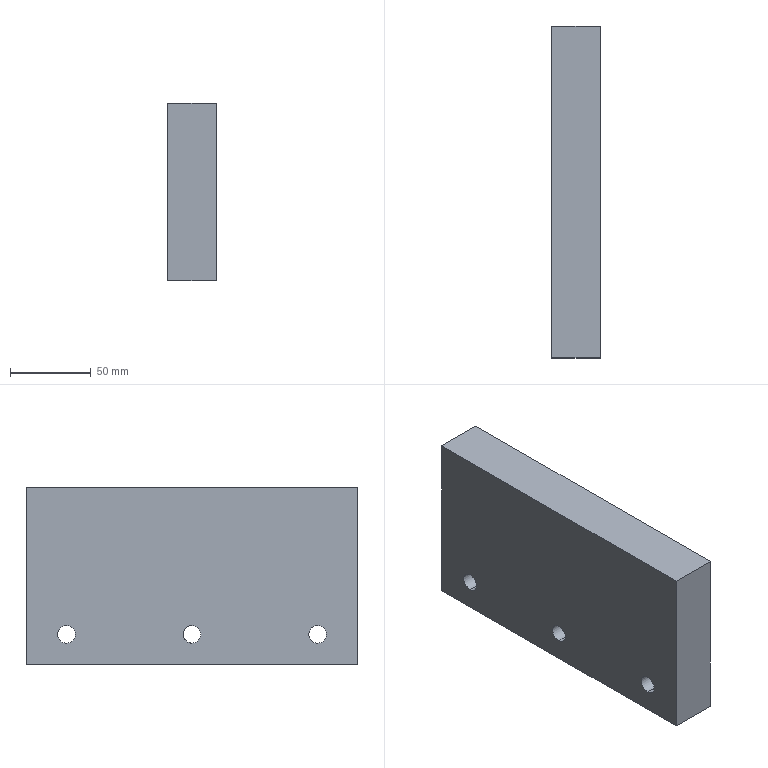Part | Creo | 1 solid | 21 faces | box 30 x 206.013 x 110.125 mm | volume 667483 mm3 | cylinder 12 | plane 9 | commonest cylinder face diameters 11 x6 17.25 x6
STEP:
#1=CARTESIAN_POINT('',(0.,0.,0.));
#2=DIRECTION('',(0.,0.,1.));
#3=DIRECTION('',(1.,0.,0.));
#4=AXIS2_PLACEMENT_3D('',#1,#2,#3);
#5=CARTESIAN_POINT('',(798.101,-95.244,-43.317));
#6=VERTEX_POINT('',#5);
#7=CARTESIAN_POINT('',(798.101,110.769,-43.317));
#8=VERTEX_POINT('',#7);
#9=CARTESIAN_POINT('',(798.101,-95.244,-43.317));
#10=DIRECTION('',(0.,1.,0.));
#11=VECTOR('',#10,206.013);
#12=LINE('',#9,#11);
#13=EDGE_CURVE('',#6,#8,#12,.T.);
#14=ORIENTED_EDGE('',*,*,#13,.T.);
#15=CARTESIAN_POINT('',(798.101,110.769,-153.441));
#16=VERTEX_POINT('',#15);
#17=CARTESIAN_POINT('',(798.101,110.769,-43.317));
#18=DIRECTION('',(0.,0.,-1.));
#19=VECTOR('',#18,110.125);
#20=LINE('',#17,#19);
#21=EDGE_CURVE('',#8,#16,#20,.T.);
#22=ORIENTED_EDGE('',*,*,#21,.T.);
#23=CARTESIAN_POINT('',(798.101,-95.244,-153.441));
#24=VERTEX_POINT('',#23);
#25=CARTESIAN_POINT('',(798.101,-95.244,-153.441));
#26=DIRECTION('',(0.,1.,0.));
#27=VECTOR('',#26,206.013);
#28=LINE('',#25,#27);
#29=EDGE_CURVE('',#24,#16,#28,.T.);
#30=ORIENTED_EDGE('',*,*,#29,.F.);
#31=CARTESIAN_POINT('',(798.101,-95.244,-43.317));
#32=DIRECTION('',(0.,0.,-1.));
#33=VECTOR('',#32,110.125);
#34=LINE('',#31,#33);
#35=EDGE_CURVE('',#6,#24,#34,.T.);
#36=ORIENTED_EDGE('',*,*,#35,.F.);
#37=EDGE_LOOP('',(#14,#22,#30,#36));
#38=FACE_OUTER_BOUND('',#37,.F.);
#39=CARTESIAN_POINT('',(798.101,16.387,-134.619));
#40=VERTEX_POINT('',#39);
#41=CARTESIAN_POINT('',(798.101,7.762,-143.244));
#42=VERTEX_POINT('',#41);
#43=CARTESIAN_POINT('',(798.101,7.762,-134.619));
#44=DIRECTION('',(-1.,0.,0.));
#45=DIRECTION('',(0.,1.,0.));
#46=AXIS2_PLACEMENT_3D('',#43,#44,#45);
#47=CIRCLE('',#46,8.625);
#48=EDGE_CURVE('',#40,#42,#47,.T.);
#49=ORIENTED_EDGE('',*,*,#48,.F.);
#50=CARTESIAN_POINT('',(798.101,7.762,-125.994));
#51=VERTEX_POINT('',#50);
#52=CARTESIAN_POINT('',(798.101,7.762,-134.619));
#53=DIRECTION('',(-1.,0.,0.));
#54=DIRECTION('',(0.,0.,1.));
#55=AXIS2_PLACEMENT_3D('',#52,#53,#54);
#56=CIRCLE('',#55,8.625);
#57=EDGE_CURVE('',#51,#40,#56,.T.);
#58=ORIENTED_EDGE('',*,*,#57,.F.);
#59=CARTESIAN_POINT('',(798.101,7.762,-134.619));
#60=DIRECTION('',(-1.,0.,0.));
#61=DIRECTION('',(0.,0.,-1.));
#62=AXIS2_PLACEMENT_3D('',#59,#60,#61);
#63=CIRCLE('',#62,8.625);
#64=EDGE_CURVE('',#42,#51,#63,.T.);
#65=ORIENTED_EDGE('',*,*,#64,.F.);
#66=EDGE_LOOP('',(#49,#58,#65));
#67=FACE_BOUND('',#66,.F.);
#68=CARTESIAN_POINT('',(798.101,94.394,-134.619));
#69=VERTEX_POINT('',#68);
#70=CARTESIAN_POINT('',(798.101,85.769,-143.244));
#71=VERTEX_POINT('',#70);
#72=CARTESIAN_POINT('',(798.101,85.769,-134.619));
#73=DIRECTION('',(-1.,0.,0.));
#74=DIRECTION('',(0.,1.,0.));
#75=AXIS2_PLACEMENT_3D('',#72,#73,#74);
#76=CIRCLE('',#75,8.625);
#77=EDGE_CURVE('',#69,#71,#76,.T.);
#78=ORIENTED_EDGE('',*,*,#77,.F.);
#79=CARTESIAN_POINT('',(798.101,85.769,-125.994));
#80=VERTEX_POINT('',#79);
#81=CARTESIAN_POINT('',(798.101,85.769,-134.619));
#82=DIRECTION('',(-1.,0.,0.));
#83=DIRECTION('',(0.,0.,1.));
#84=AXIS2_PLACEMENT_3D('',#81,#82,#83);
#85=CIRCLE('',#84,8.625);
#86=EDGE_CURVE('',#80,#69,#85,.T.);
#87=ORIENTED_EDGE('',*,*,#86,.F.);
#88=CARTESIAN_POINT('',(798.101,85.769,-134.619));
#89=DIRECTION('',(-1.,0.,0.));
#90=DIRECTION('',(0.,0.,-1.));
#91=AXIS2_PLACEMENT_3D('',#88,#89,#90);
#92=CIRCLE('',#91,8.625);
#93=EDGE_CURVE('',#71,#80,#92,.T.);
#94=ORIENTED_EDGE('',*,*,#93,.F.);
#95=EDGE_LOOP('',(#78,#87,#94));
#96=FACE_BOUND('',#95,.F.);
#97=CARTESIAN_POINT('',(798.101,-61.619,-134.619));
#98=VERTEX_POINT('',#97);
#99=CARTESIAN_POINT('',(798.101,-70.244,-143.244));
#100=VERTEX_POINT('',#99);
#101=CARTESIAN_POINT('',(798.101,-70.244,-134.619));
#102=DIRECTION('',(-1.,0.,0.));
#103=DIRECTION('',(0.,1.,0.));
#104=AXIS2_PLACEMENT_3D('',#101,#102,#103);
#105=CIRCLE('',#104,8.625);
#106=EDGE_CURVE('',#98,#100,#105,.T.);
#107=ORIENTED_EDGE('',*,*,#106,.F.);
#108=CARTESIAN_POINT('',(798.101,-70.244,-125.994));
#109=VERTEX_POINT('',#108);
#110=CARTESIAN_POINT('',(798.101,-70.244,-134.619));
#111=DIRECTION('',(-1.,0.,0.));
#112=DIRECTION('',(0.,0.,1.));
#113=AXIS2_PLACEMENT_3D('',#110,#111,#112);
#114=CIRCLE('',#113,8.625);
#115=EDGE_CURVE('',#109,#98,#114,.T.);
#116=ORIENTED_EDGE('',*,*,#115,.F.);
#117=CARTESIAN_POINT('',(798.101,-70.244,-134.619));
#118=DIRECTION('',(-1.,0.,0.));
#119=DIRECTION('',(0.,0.,-1.));
#120=AXIS2_PLACEMENT_3D('',#117,#118,#119);
#121=CIRCLE('',#120,8.625);
#122=EDGE_CURVE('',#100,#109,#121,.T.);
#123=ORIENTED_EDGE('',*,*,#122,.F.);
#124=EDGE_LOOP('',(#107,#116,#123));
#125=FACE_BOUND('',#124,.F.);
#126=CARTESIAN_POINT('',(798.101,8.76,-121.835));
#127=DIRECTION('',(-1.,0.,0.));
#128=DIRECTION('',(0.,0.,1.));
#129=AXIS2_PLACEMENT_3D('',#126,#127,#128);
#130=PLANE('',#129);
#131=ADVANCED_FACE('',(#38,#67,#96,#125),#130,.F.);
#132=ORIENTED_EDGE('',*,*,#57,.T.);
#133=ORIENTED_EDGE('',*,*,#48,.T.);
#134=CARTESIAN_POINT('',(787.101,7.762,-143.244));
#135=VERTEX_POINT('',#134);
#136=CARTESIAN_POINT('',(787.101,7.762,-143.244));
#137=DIRECTION('',(1.,0.,0.));
#138=VECTOR('',#137,11.);
#139=LINE('',#136,#138);
#140=EDGE_CURVE('',#135,#42,#139,.T.);
#141=ORIENTED_EDGE('',*,*,#140,.F.);
#142=CARTESIAN_POINT('',(787.101,16.387,-134.619));
#143=VERTEX_POINT('',#142);
#144=CARTESIAN_POINT('',(787.101,7.762,-134.619));
#145=DIRECTION('',(1.,0.,0.));
#146=DIRECTION('',(0.,0.,-1.));
#147=AXIS2_PLACEMENT_3D('',#144,#145,#146);
#148=CIRCLE('',#147,8.625);
#149=EDGE_CURVE('',#135,#143,#148,.T.);
#150=ORIENTED_EDGE('',*,*,#149,.T.);
#151=CARTESIAN_POINT('',(787.101,7.762,-125.994));
#152=VERTEX_POINT('',#151);
#153=CARTESIAN_POINT('',(787.101,7.762,-134.619));
#154=DIRECTION('',(1.,0.,0.));
#155=DIRECTION('',(0.,1.,0.));
#156=AXIS2_PLACEMENT_3D('',#153,#154,#155);
#157=CIRCLE('',#156,8.625);
#158=EDGE_CURVE('',#143,#152,#157,.T.);
#159=ORIENTED_EDGE('',*,*,#158,.T.);
#160=CARTESIAN_POINT('',(787.101,7.762,-125.994));
#161=DIRECTION('',(1.,0.,0.));
#162=VECTOR('',#161,11.);
#163=LINE('',#160,#162);
#164=EDGE_CURVE('',#152,#51,#163,.T.);
#165=ORIENTED_EDGE('',*,*,#164,.T.);
#166=EDGE_LOOP('',(#132,#133,#141,#150,#159,#165));
#167=FACE_OUTER_BOUND('',#166,.F.);
#168=CARTESIAN_POINT('',(787.101,7.762,-134.619));
#169=DIRECTION('',(1.,0.,0.));
#170=DIRECTION('',(0.,0.,-1.));
#171=AXIS2_PLACEMENT_3D('',#168,#169,#170);
#172=CYLINDRICAL_SURFACE('',#171,8.625);
#173=ADVANCED_FACE('',(#167),#172,.F.);
#174=ORIENTED_EDGE('',*,*,#64,.T.);
#175=ORIENTED_EDGE('',*,*,#164,.F.);
#176=CARTESIAN_POINT('',(787.101,-0.8626,-134.619));
#177=VERTEX_POINT('',#176);
#178=CARTESIAN_POINT('',(787.101,7.762,-134.619));
#179=DIRECTION('',(1.,0.,0.));
#180=DIRECTION('',(0.,0.,1.));
#181=AXIS2_PLACEMENT_3D('',#178,#179,#180);
#182=CIRCLE('',#181,8.625);
#183=EDGE_CURVE('',#152,#177,#182,.T.);
#184=ORIENTED_EDGE('',*,*,#183,.T.);
#185=CARTESIAN_POINT('',(787.101,7.762,-134.619));
#186=DIRECTION('',(1.,0.,0.));
#187=DIRECTION('',(0.,-1.,0.));
#188=AXIS2_PLACEMENT_3D('',#185,#186,#187);
#189=CIRCLE('',#188,8.625);
#190=EDGE_CURVE('',#177,#135,#189,.T.);
#191=ORIENTED_EDGE('',*,*,#190,.T.);
#192=ORIENTED_EDGE('',*,*,#140,.T.);
#193=EDGE_LOOP('',(#174,#175,#184,#191,#192));
#194=FACE_OUTER_BOUND('',#193,.F.);
#195=CARTESIAN_POINT('',(787.101,7.762,-134.619));
#196=DIRECTION('',(1.,0.,0.));
#197=DIRECTION('',(0.,0.,-1.));
#198=AXIS2_PLACEMENT_3D('',#195,#196,#197);
#199=CYLINDRICAL_SURFACE('',#198,8.625);
#200=ADVANCED_FACE('',(#194),#199,.F.);
#201=ORIENTED_EDGE('',*,*,#158,.F.);
#202=ORIENTED_EDGE('',*,*,#149,.F.);
#203=ORIENTED_EDGE('',*,*,#190,.F.);
#204=ORIENTED_EDGE('',*,*,#183,.F.);
#205=EDGE_LOOP('',(#201,#202,#203,#204));
#206=FACE_OUTER_BOUND('',#205,.F.);
#207=CARTESIAN_POINT('',(787.101,2.262,-134.619));
#208=VERTEX_POINT('',#207);
#209=CARTESIAN_POINT('',(787.101,7.762,-129.119));
#210=VERTEX_POINT('',#209);
#211=CARTESIAN_POINT('',(787.101,7.762,-134.619));
#212=DIRECTION('',(-1.,0.,0.));
#213=DIRECTION('',(0.,-1.,0.));
#214=AXIS2_PLACEMENT_3D('',#211,#212,#213);
#215=CIRCLE('',#214,5.5);
#216=EDGE_CURVE('',#208,#210,#215,.T.);
#217=ORIENTED_EDGE('',*,*,#216,.F.);
#218=CARTESIAN_POINT('',(787.101,7.762,-140.119));
#219=VERTEX_POINT('',#218);
#220=CARTESIAN_POINT('',(787.101,7.762,-134.619));
#221=DIRECTION('',(-1.,0.,0.));
#222=DIRECTION('',(0.,0.,-1.));
#223=AXIS2_PLACEMENT_3D('',#220,#221,#222);
#224=CIRCLE('',#223,5.5);
#225=EDGE_CURVE('',#219,#208,#224,.T.);
#226=ORIENTED_EDGE('',*,*,#225,.F.);
#227=CARTESIAN_POINT('',(787.101,13.262,-134.619));
#228=VERTEX_POINT('',#227);
#229=CARTESIAN_POINT('',(787.101,7.762,-134.619));
#230=DIRECTION('',(-1.,0.,0.));
#231=DIRECTION('',(0.,1.,0.));
#232=AXIS2_PLACEMENT_3D('',#229,#230,#231);
#233=CIRCLE('',#232,5.5);
#234=EDGE_CURVE('',#228,#219,#233,.T.);
#235=ORIENTED_EDGE('',*,*,#234,.F.);
#236=CARTESIAN_POINT('',(787.101,7.762,-134.619));
#237=DIRECTION('',(-1.,0.,0.));
#238=DIRECTION('',(0.,0.,1.));
#239=AXIS2_PLACEMENT_3D('',#236,#237,#238);
#240=CIRCLE('',#239,5.5);
#241=EDGE_CURVE('',#210,#228,#240,.T.);
#242=ORIENTED_EDGE('',*,*,#241,.F.);
#243=EDGE_LOOP('',(#217,#226,#235,#242));
#244=FACE_BOUND('',#243,.F.);
#245=CARTESIAN_POINT('',(787.101,7.762,-134.619));
#246=DIRECTION('',(-1.,0.,0.));
#247=DIRECTION('',(0.,0.,1.));
#248=AXIS2_PLACEMENT_3D('',#245,#246,#247);
#249=PLANE('',#248);
#250=ADVANCED_FACE('',(#206,#244),#249,.F.);
#251=CARTESIAN_POINT('',(768.101,7.762,-129.119));
#252=VERTEX_POINT('',#251);
#253=CARTESIAN_POINT('',(768.101,2.262,-134.619));
#254=VERTEX_POINT('',#253);
#255=CARTESIAN_POINT('',(768.101,7.762,-134.619));
#256=DIRECTION('',(1.,0.,0.));
#257=DIRECTION('',(0.,0.,1.));
#258=AXIS2_PLACEMENT_3D('',#255,#256,#257);
#259=CIRCLE('',#258,5.5);
#260=EDGE_CURVE('',#252,#254,#259,.T.);
#261=ORIENTED_EDGE('',*,*,#260,.T.);
#262=CARTESIAN_POINT('',(768.101,7.762,-140.119));
#263=VERTEX_POINT('',#262);
#264=CARTESIAN_POINT('',(768.101,7.762,-134.619));
#265=DIRECTION('',(1.,0.,0.));
#266=DIRECTION('',(0.,-1.,0.));
#267=AXIS2_PLACEMENT_3D('',#264,#265,#266);
#268=CIRCLE('',#267,5.5);
#269=EDGE_CURVE('',#254,#263,#268,.T.);
#270=ORIENTED_EDGE('',*,*,#269,.T.);
#271=CARTESIAN_POINT('',(787.101,7.762,-140.119));
#272=DIRECTION('',(-1.,0.,0.));
#273=VECTOR('',#272,19.);
#274=LINE('',#271,#273);
#275=EDGE_CURVE('',#219,#263,#274,.T.);
#276=ORIENTED_EDGE('',*,*,#275,.F.);
#277=ORIENTED_EDGE('',*,*,#225,.T.);
#278=ORIENTED_EDGE('',*,*,#216,.T.);
#279=CARTESIAN_POINT('',(787.101,7.762,-129.119));
#280=DIRECTION('',(-1.,0.,0.));
#281=VECTOR('',#280,19.);
#282=LINE('',#279,#281);
#283=EDGE_CURVE('',#210,#252,#282,.T.);
#284=ORIENTED_EDGE('',*,*,#283,.T.);
#285=EDGE_LOOP('',(#261,#270,#276,#277,#278,#284));
#286=FACE_OUTER_BOUND('',#285,.F.);
#287=CARTESIAN_POINT('',(787.101,7.762,-134.619));
#288=DIRECTION('',(-1.,0.,0.));
#289=DIRECTION('',(0.,0.,1.));
#290=AXIS2_PLACEMENT_3D('',#287,#288,#289);
#291=CYLINDRICAL_SURFACE('',#290,5.5);
#292=ADVANCED_FACE('',(#286),#291,.F.);
#293=CARTESIAN_POINT('',(768.101,-95.244,-43.317));
#294=VERTEX_POINT('',#293);
#295=CARTESIAN_POINT('',(768.101,-95.244,-153.441));
#296=VERTEX_POINT('',#295);
#297=CARTESIAN_POINT('',(768.101,-95.244,-43.317));
#298=DIRECTION('',(0.,0.,-1.));
#299=VECTOR('',#298,110.125);
#300=LINE('',#297,#299);
#301=EDGE_CURVE('',#294,#296,#300,.T.);
#302=ORIENTED_EDGE('',*,*,#301,.T.);
#303=CARTESIAN_POINT('',(768.101,110.769,-153.441));
#304=VERTEX_POINT('',#303);
#305=CARTESIAN_POINT('',(768.101,-95.244,-153.441));
#306=DIRECTION('',(0.,1.,0.));
#307=VECTOR('',#306,206.013);
#308=LINE('',#305,#307);
#309=EDGE_CURVE('',#296,#304,#308,.T.);
#310=ORIENTED_EDGE('',*,*,#309,.T.);
#311=CARTESIAN_POINT('',(768.101,110.769,-43.317));
#312=VERTEX_POINT('',#311);
#313=CARTESIAN_POINT('',(768.101,110.769,-43.317));
#314=DIRECTION('',(0.,0.,-1.));
#315=VECTOR('',#314,110.125);
#316=LINE('',#313,#315);
#317=EDGE_CURVE('',#312,#304,#316,.T.);
#318=ORIENTED_EDGE('',*,*,#317,.F.);
#319=CARTESIAN_POINT('',(768.101,-95.244,-43.317));
#320=DIRECTION('',(0.,1.,0.));
#321=VECTOR('',#320,206.013);
#322=LINE('',#319,#321);
#323=EDGE_CURVE('',#294,#312,#322,.T.);
#324=ORIENTED_EDGE('',*,*,#323,.F.);
#325=EDGE_LOOP('',(#302,#310,#318,#324));
#326=FACE_OUTER_BOUND('',#325,.F.);
#327=ORIENTED_EDGE('',*,*,#269,.F.);
#328=ORIENTED_EDGE('',*,*,#260,.F.);
#329=CARTESIAN_POINT('',(768.101,7.762,-134.619));
#330=DIRECTION('',(1.,0.,0.));
#331=DIRECTION('',(0.,0.,-1.));
#332=AXIS2_PLACEMENT_3D('',#329,#330,#331);
#333=CIRCLE('',#332,5.5);
#334=EDGE_CURVE('',#263,#252,#333,.T.);
#335=ORIENTED_EDGE('',*,*,#334,.F.);
#336=EDGE_LOOP('',(#327,#328,#335));
#337=FACE_BOUND('',#336,.F.);
#338=CARTESIAN_POINT('',(768.101,80.269,-134.619));
#339=VERTEX_POINT('',#338);
#340=CARTESIAN_POINT('',(768.101,85.769,-140.119));
#341=VERTEX_POINT('',#340);
#342=CARTESIAN_POINT('',(768.101,85.769,-134.619));
#343=DIRECTION('',(1.,0.,0.));
#344=DIRECTION('',(0.,-1.,0.));
#345=AXIS2_PLACEMENT_3D('',#342,#343,#344);
#346=CIRCLE('',#345,5.5);
#347=EDGE_CURVE('',#339,#341,#346,.T.);
#348=ORIENTED_EDGE('',*,*,#347,.F.);
#349=CARTESIAN_POINT('',(768.101,85.769,-129.119));
#350=VERTEX_POINT('',#349);
#351=CARTESIAN_POINT('',(768.101,85.769,-134.619));
#352=DIRECTION('',(1.,0.,0.));
#353=DIRECTION('',(0.,0.,1.));
#354=AXIS2_PLACEMENT_3D('',#351,#352,#353);
#355=CIRCLE('',#354,5.5);
#356=EDGE_CURVE('',#350,#339,#355,.T.);
#357=ORIENTED_EDGE('',*,*,#356,.F.);
#358=CARTESIAN_POINT('',(768.101,85.769,-134.619));
#359=DIRECTION('',(1.,0.,0.));
#360=DIRECTION('',(0.,0.,-1.));
#361=AXIS2_PLACEMENT_3D('',#358,#359,#360);
#362=CIRCLE('',#361,5.5);
#363=EDGE_CURVE('',#341,#350,#362,.T.);
#364=ORIENTED_EDGE('',*,*,#363,.F.);
#365=EDGE_LOOP('',(#348,#357,#364));
#366=FACE_BOUND('',#365,.F.);
#367=CARTESIAN_POINT('',(768.101,-75.744,-134.619));
#368=VERTEX_POINT('',#367);
#369=CARTESIAN_POINT('',(768.101,-70.244,-140.119));
#370=VERTEX_POINT('',#369);
#371=CARTESIAN_POINT('',(768.101,-70.244,-134.619));
#372=DIRECTION('',(1.,0.,0.));
#373=DIRECTION('',(0.,-1.,0.));
#374=AXIS2_PLACEMENT_3D('',#371,#372,#373);
#375=CIRCLE('',#374,5.5);
#376=EDGE_CURVE('',#368,#370,#375,.T.);
#377=ORIENTED_EDGE('',*,*,#376,.F.);
#378=CARTESIAN_POINT('',(768.101,-70.244,-129.119));
#379=VERTEX_POINT('',#378);
#380=CARTESIAN_POINT('',(768.101,-70.244,-134.619));
#381=DIRECTION('',(1.,0.,0.));
#382=DIRECTION('',(0.,0.,1.));
#383=AXIS2_PLACEMENT_3D('',#380,#381,#382);
#384=CIRCLE('',#383,5.5);
#385=EDGE_CURVE('',#379,#368,#384,.T.);
#386=ORIENTED_EDGE('',*,*,#385,.F.);
#387=CARTESIAN_POINT('',(768.101,-70.244,-134.619));
#388=DIRECTION('',(1.,0.,0.));
#389=DIRECTION('',(0.,0.,-1.));
#390=AXIS2_PLACEMENT_3D('',#387,#388,#389);
#391=CIRCLE('',#390,5.5);
#392=EDGE_CURVE('',#370,#379,#391,.T.);
#393=ORIENTED_EDGE('',*,*,#392,.F.);
#394=EDGE_LOOP('',(#377,#386,#393));
#395=FACE_BOUND('',#394,.F.);
#396=CARTESIAN_POINT('',(768.101,8.76,-121.835));
#397=DIRECTION('',(-1.,0.,0.));
#398=DIRECTION('',(0.,0.,1.));
#399=AXIS2_PLACEMENT_3D('',#396,#397,#398);
#400=PLANE('',#399);
#401=ADVANCED_FACE('',(#326,#337,#366,#395),#400,.T.);
#402=ORIENTED_EDGE('',*,*,#385,.T.);
#403=ORIENTED_EDGE('',*,*,#376,.T.);
#404=CARTESIAN_POINT('',(787.101,-70.244,-140.119));
#405=VERTEX_POINT('',#404);
#406=CARTESIAN_POINT('',(787.101,-70.244,-140.119));
#407=DIRECTION('',(-1.,0.,0.));
#408=VECTOR('',#407,19.);
#409=LINE('',#406,#408);
#410=EDGE_CURVE('',#405,#370,#409,.T.);
#411=ORIENTED_EDGE('',*,*,#410,.F.);
#412=CARTESIAN_POINT('',(787.101,-75.744,-134.619));
#413=VERTEX_POINT('',#412);
#414=CARTESIAN_POINT('',(787.101,-70.244,-134.619));
#415=DIRECTION('',(-1.,0.,0.));
#416=DIRECTION('',(0.,0.,-1.));
#417=AXIS2_PLACEMENT_3D('',#414,#415,#416);
#418=CIRCLE('',#417,5.5);
#419=EDGE_CURVE('',#405,#413,#418,.T.);
#420=ORIENTED_EDGE('',*,*,#419,.T.);
#421=CARTESIAN_POINT('',(787.101,-70.244,-129.119));
#422=VERTEX_POINT('',#421);
#423=CARTESIAN_POINT('',(787.101,-70.244,-134.619));
#424=DIRECTION('',(-1.,0.,0.));
#425=DIRECTION('',(0.,-1.,0.));
#426=AXIS2_PLACEMENT_3D('',#423,#424,#425);
#427=CIRCLE('',#426,5.5);
#428=EDGE_CURVE('',#413,#422,#427,.T.);
#429=ORIENTED_EDGE('',*,*,#428,.T.);
#430=CARTESIAN_POINT('',(787.101,-70.244,-129.119));
#431=DIRECTION('',(-1.,0.,0.));
#432=VECTOR('',#431,19.);
#433=LINE('',#430,#432);
#434=EDGE_CURVE('',#422,#379,#433,.T.);
#435=ORIENTED_EDGE('',*,*,#434,.T.);
#436=EDGE_LOOP('',(#402,#403,#411,#420,#429,#435));
#437=FACE_OUTER_BOUND('',#436,.F.);
#438=CARTESIAN_POINT('',(787.101,-70.244,-134.619));
#439=DIRECTION('',(-1.,0.,0.));
#440=DIRECTION('',(0.,0.,1.));
#441=AXIS2_PLACEMENT_3D('',#438,#439,#440);
#442=CYLINDRICAL_SURFACE('',#441,5.5);
#443=ADVANCED_FACE('',(#437),#442,.F.);
#444=ORIENTED_EDGE('',*,*,#392,.T.);
#445=ORIENTED_EDGE('',*,*,#434,.F.);
#446=CARTESIAN_POINT('',(787.101,-64.744,-134.619));
#447=VERTEX_POINT('',#446);
#448=CARTESIAN_POINT('',(787.101,-70.244,-134.619));
#449=DIRECTION('',(-1.,0.,0.));
#450=DIRECTION('',(0.,0.,1.));
#451=AXIS2_PLACEMENT_3D('',#448,#449,#450);
#452=CIRCLE('',#451,5.5);
#453=EDGE_CURVE('',#422,#447,#452,.T.);
#454=ORIENTED_EDGE('',*,*,#453,.T.);
#455=CARTESIAN_POINT('',(787.101,-70.244,-134.619));
#456=DIRECTION('',(-1.,0.,0.));
#457=DIRECTION('',(0.,1.,0.));
#458=AXIS2_PLACEMENT_3D('',#455,#456,#457);
#459=CIRCLE('',#458,5.5);
#460=EDGE_CURVE('',#447,#405,#459,.T.);
#461=ORIENTED_EDGE('',*,*,#460,.T.);
#462=ORIENTED_EDGE('',*,*,#410,.T.);
#463=EDGE_LOOP('',(#444,#445,#454,#461,#462));
#464=FACE_OUTER_BOUND('',#463,.F.);
#465=CARTESIAN_POINT('',(787.101,-70.244,-134.619));
#466=DIRECTION('',(-1.,0.,0.));
#467=DIRECTION('',(0.,0.,1.));
#468=AXIS2_PLACEMENT_3D('',#465,#466,#467);
#469=CYLINDRICAL_SURFACE('',#468,5.5);
#470=ADVANCED_FACE('',(#464),#469,.F.);
#471=CARTESIAN_POINT('',(787.101,-61.619,-134.619));
#472=VERTEX_POINT('',#471);
#473=CARTESIAN_POINT('',(787.101,-70.244,-125.994));
#474=VERTEX_POINT('',#473);
#475=CARTESIAN_POINT('',(787.101,-70.244,-134.619));
#476=DIRECTION('',(1.,0.,0.));
#477=DIRECTION('',(0.,1.,0.));
#478=AXIS2_PLACEMENT_3D('',#475,#476,#477);
#479=CIRCLE('',#478,8.625);
#480=EDGE_CURVE('',#472,#474,#479,.T.);
#481=ORIENTED_EDGE('',*,*,#480,.F.);
#482=CARTESIAN_POINT('',(787.101,-70.244,-143.244));
#483=VERTEX_POINT('',#482);
#484=CARTESIAN_POINT('',(787.101,-70.244,-134.619));
#485=DIRECTION('',(1.,0.,0.));
#486=DIRECTION('',(0.,0.,-1.));
#487=AXIS2_PLACEMENT_3D('',#484,#485,#486);
#488=CIRCLE('',#487,8.625);
#489=EDGE_CURVE('',#483,#472,#488,.T.);
#490=ORIENTED_EDGE('',*,*,#489,.F.);
#491=CARTESIAN_POINT('',(787.101,-78.869,-134.619));
#492=VERTEX_POINT('',#491);
#493=CARTESIAN_POINT('',(787.101,-70.244,-134.619));
#494=DIRECTION('',(1.,0.,0.));
#495=DIRECTION('',(0.,-1.,0.));
#496=AXIS2_PLACEMENT_3D('',#493,#494,#495);
#497=CIRCLE('',#496,8.625);
#498=EDGE_CURVE('',#492,#483,#497,.T.);
#499=ORIENTED_EDGE('',*,*,#498,.F.);
#500=CARTESIAN_POINT('',(787.101,-70.244,-134.619));
#501=DIRECTION('',(1.,0.,0.));
#502=DIRECTION('',(0.,0.,1.));
#503=AXIS2_PLACEMENT_3D('',#500,#501,#502);
#504=CIRCLE('',#503,8.625);
#505=EDGE_CURVE('',#474,#492,#504,.T.);
#506=ORIENTED_EDGE('',*,*,#505,.F.);
#507=EDGE_LOOP('',(#481,#490,#499,#506));
#508=FACE_OUTER_BOUND('',#507,.F.);
#509=ORIENTED_EDGE('',*,*,#428,.F.);
#510=ORIENTED_EDGE('',*,*,#419,.F.);
#511=ORIENTED_EDGE('',*,*,#460,.F.);
#512=ORIENTED_EDGE('',*,*,#453,.F.);
#513=EDGE_LOOP('',(#509,#510,#511,#512));
#514=FACE_BOUND('',#513,.F.);
#515=CARTESIAN_POINT('',(787.101,-70.244,-134.619));
#516=DIRECTION('',(-1.,0.,0.));
#517=DIRECTION('',(0.,0.,1.));
#518=AXIS2_PLACEMENT_3D('',#515,#516,#517);
#519=PLANE('',#518);
#520=ADVANCED_FACE('',(#508,#514),#519,.F.);
#521=ORIENTED_EDGE('',*,*,#115,.T.);
#522=ORIENTED_EDGE('',*,*,#106,.T.);
#523=CARTESIAN_POINT('',(787.101,-70.244,-143.244));
#524=DIRECTION('',(1.,0.,0.));
#525=VECTOR('',#524,11.);
#526=LINE('',#523,#525);
#527=EDGE_CURVE('',#483,#100,#526,.T.);
#528=ORIENTED_EDGE('',*,*,#527,.F.);
#529=ORIENTED_EDGE('',*,*,#489,.T.);
#530=ORIENTED_EDGE('',*,*,#480,.T.);
#531=CARTESIAN_POINT('',(787.101,-70.244,-125.994));
#532=DIRECTION('',(1.,0.,0.));
#533=VECTOR('',#532,11.);
#534=LINE('',#531,#533);
#535=EDGE_CURVE('',#474,#109,#534,.T.);
#536=ORIENTED_EDGE('',*,*,#535,.T.);
#537=EDGE_LOOP('',(#521,#522,#528,#529,#530,#536));
#538=FACE_OUTER_BOUND('',#537,.F.);
#539=CARTESIAN_POINT('',(787.101,-70.244,-134.619));
#540=DIRECTION('',(1.,0.,0.));
#541=DIRECTION('',(0.,0.,-1.));
#542=AXIS2_PLACEMENT_3D('',#539,#540,#541);
#543=CYLINDRICAL_SURFACE('',#542,8.625);
#544=ADVANCED_FACE('',(#538),#543,.F.);
#545=ORIENTED_EDGE('',*,*,#122,.T.);
#546=ORIENTED_EDGE('',*,*,#535,.F.);
#547=ORIENTED_EDGE('',*,*,#505,.T.);
#548=ORIENTED_EDGE('',*,*,#498,.T.);
#549=ORIENTED_EDGE('',*,*,#527,.T.);
#550=EDGE_LOOP('',(#545,#546,#547,#548,#549));
#551=FACE_OUTER_BOUND('',#550,.F.);
#552=CARTESIAN_POINT('',(787.101,-70.244,-134.619));
#553=DIRECTION('',(1.,0.,0.));
#554=DIRECTION('',(0.,0.,-1.));
#555=AXIS2_PLACEMENT_3D('',#552,#553,#554);
#556=CYLINDRICAL_SURFACE('',#555,8.625);
#557=ADVANCED_FACE('',(#551),#556,.F.);
#558=ORIENTED_EDGE('',*,*,#334,.T.);
#559=ORIENTED_EDGE('',*,*,#283,.F.);
#560=ORIENTED_EDGE('',*,*,#241,.T.);
#561=ORIENTED_EDGE('',*,*,#234,.T.);
#562=ORIENTED_EDGE('',*,*,#275,.T.);
#563=EDGE_LOOP('',(#558,#559,#560,#561,#562));
#564=FACE_OUTER_BOUND('',#563,.F.);
#565=CARTESIAN_POINT('',(787.101,7.762,-134.619));
#566=DIRECTION('',(-1.,0.,0.));
#567=DIRECTION('',(0.,0.,1.));
#568=AXIS2_PLACEMENT_3D('',#565,#566,#567);
#569=CYLINDRICAL_SURFACE('',#568,5.5);
#570=ADVANCED_FACE('',(#564),#569,.F.);
#571=ORIENTED_EDGE('',*,*,#356,.T.);
#572=ORIENTED_EDGE('',*,*,#347,.T.);
#573=CARTESIAN_POINT('',(787.101,85.769,-140.119));
#574=VERTEX_POINT('',#573);
#575=CARTESIAN_POINT('',(787.101,85.769,-140.119));
#576=DIRECTION('',(-1.,0.,0.));
#577=VECTOR('',#576,19.);
#578=LINE('',#575,#577);
#579=EDGE_CURVE('',#574,#341,#578,.T.);
#580=ORIENTED_EDGE('',*,*,#579,.F.);
#581=CARTESIAN_POINT('',(787.101,80.269,-134.619));
#582=VERTEX_POINT('',#581);
#583=CARTESIAN_POINT('',(787.101,85.769,-134.619));
#584=DIRECTION('',(-1.,0.,0.));
#585=DIRECTION('',(0.,0.,-1.));
#586=AXIS2_PLACEMENT_3D('',#583,#584,#585);
#587=CIRCLE('',#586,5.5);
#588=EDGE_CURVE('',#574,#582,#587,.T.);
#589=ORIENTED_EDGE('',*,*,#588,.T.);
#590=CARTESIAN_POINT('',(787.101,85.769,-129.119));
#591=VERTEX_POINT('',#590);
#592=CARTESIAN_POINT('',(787.101,85.769,-134.619));
#593=DIRECTION('',(-1.,0.,0.));
#594=DIRECTION('',(0.,-1.,0.));
#595=AXIS2_PLACEMENT_3D('',#592,#593,#594);
#596=CIRCLE('',#595,5.5);
#597=EDGE_CURVE('',#582,#591,#596,.T.);
#598=ORIENTED_EDGE('',*,*,#597,.T.);
#599=CARTESIAN_POINT('',(787.101,85.769,-129.119));
#600=DIRECTION('',(-1.,0.,0.));
#601=VECTOR('',#600,19.);
#602=LINE('',#599,#601);
#603=EDGE_CURVE('',#591,#350,#602,.T.);
#604=ORIENTED_EDGE('',*,*,#603,.T.);
#605=EDGE_LOOP('',(#571,#572,#580,#589,#598,#604));
#606=FACE_OUTER_BOUND('',#605,.F.);
#607=CARTESIAN_POINT('',(787.101,85.769,-134.619));
#608=DIRECTION('',(-1.,0.,0.));
#609=DIRECTION('',(0.,0.,1.));
#610=AXIS2_PLACEMENT_3D('',#607,#608,#609);
#611=CYLINDRICAL_SURFACE('',#610,5.5);
#612=ADVANCED_FACE('',(#606),#611,.F.);
#613=ORIENTED_EDGE('',*,*,#363,.T.);
#614=ORIENTED_EDGE('',*,*,#603,.F.);
#615=CARTESIAN_POINT('',(787.101,91.269,-134.619));
#616=VERTEX_POINT('',#615);
#617=CARTESIAN_POINT('',(787.101,85.769,-134.619));
#618=DIRECTION('',(-1.,0.,0.));
#619=DIRECTION('',(0.,0.,1.));
#620=AXIS2_PLACEMENT_3D('',#617,#618,#619);
#621=CIRCLE('',#620,5.5);
#622=EDGE_CURVE('',#591,#616,#621,.T.);
#623=ORIENTED_EDGE('',*,*,#622,.T.);
#624=CARTESIAN_POINT('',(787.101,85.769,-134.619));
#625=DIRECTION('',(-1.,0.,0.));
#626=DIRECTION('',(0.,1.,0.));
#627=AXIS2_PLACEMENT_3D('',#624,#625,#626);
#628=CIRCLE('',#627,5.5);
#629=EDGE_CURVE('',#616,#574,#628,.T.);
#630=ORIENTED_EDGE('',*,*,#629,.T.);
#631=ORIENTED_EDGE('',*,*,#579,.T.);
#632=EDGE_LOOP('',(#613,#614,#623,#630,#631));
#633=FACE_OUTER_BOUND('',#632,.F.);
#634=CARTESIAN_POINT('',(787.101,85.769,-134.619));
#635=DIRECTION('',(-1.,0.,0.));
#636=DIRECTION('',(0.,0.,1.));
#637=AXIS2_PLACEMENT_3D('',#634,#635,#636);
#638=CYLINDRICAL_SURFACE('',#637,5.5);
#639=ADVANCED_FACE('',(#633),#638,.F.);
#640=CARTESIAN_POINT('',(787.101,94.394,-134.619));
#641=VERTEX_POINT('',#640);
#642=CARTESIAN_POINT('',(787.101,85.769,-125.994));
#643=VERTEX_POINT('',#642);
#644=CARTESIAN_POINT('',(787.101,85.769,-134.619));
#645=DIRECTION('',(1.,0.,0.));
#646=DIRECTION('',(0.,1.,0.));
#647=AXIS2_PLACEMENT_3D('',#644,#645,#646);
#648=CIRCLE('',#647,8.625);
#649=EDGE_CURVE('',#641,#643,#648,.T.);
#650=ORIENTED_EDGE('',*,*,#649,.F.);
#651=CARTESIAN_POINT('',(787.101,85.769,-143.244));
#652=VERTEX_POINT('',#651);
#653=CARTESIAN_POINT('',(787.101,85.769,-134.619));
#654=DIRECTION('',(1.,0.,0.));
#655=DIRECTION('',(0.,0.,-1.));
#656=AXIS2_PLACEMENT_3D('',#653,#654,#655);
#657=CIRCLE('',#656,8.625);
#658=EDGE_CURVE('',#652,#641,#657,.T.);
#659=ORIENTED_EDGE('',*,*,#658,.F.);
#660=CARTESIAN_POINT('',(787.101,77.144,-134.619));
#661=VERTEX_POINT('',#660);
#662=CARTESIAN_POINT('',(787.101,85.769,-134.619));
#663=DIRECTION('',(1.,0.,0.));
#664=DIRECTION('',(0.,-1.,0.));
#665=AXIS2_PLACEMENT_3D('',#662,#663,#664);
#666=CIRCLE('',#665,8.625);
#667=EDGE_CURVE('',#661,#652,#666,.T.);
#668=ORIENTED_EDGE('',*,*,#667,.F.);
#669=CARTESIAN_POINT('',(787.101,85.769,-134.619));
#670=DIRECTION('',(1.,0.,0.));
#671=DIRECTION('',(0.,0.,1.));
#672=AXIS2_PLACEMENT_3D('',#669,#670,#671);
#673=CIRCLE('',#672,8.625);
#674=EDGE_CURVE('',#643,#661,#673,.T.);
#675=ORIENTED_EDGE('',*,*,#674,.F.);
#676=EDGE_LOOP('',(#650,#659,#668,#675));
#677=FACE_OUTER_BOUND('',#676,.F.);
#678=ORIENTED_EDGE('',*,*,#597,.F.);
#679=ORIENTED_EDGE('',*,*,#588,.F.);
#680=ORIENTED_EDGE('',*,*,#629,.F.);
#681=ORIENTED_EDGE('',*,*,#622,.F.);
#682=EDGE_LOOP('',(#678,#679,#680,#681));
#683=FACE_BOUND('',#682,.F.);
#684=CARTESIAN_POINT('',(787.101,85.769,-134.619));
#685=DIRECTION('',(-1.,0.,0.));
#686=DIRECTION('',(0.,0.,1.));
#687=AXIS2_PLACEMENT_3D('',#684,#685,#686);
#688=PLANE('',#687);
#689=ADVANCED_FACE('',(#677,#683),#688,.F.);
#690=ORIENTED_EDGE('',*,*,#86,.T.);
#691=ORIENTED_EDGE('',*,*,#77,.T.);
#692=CARTESIAN_POINT('',(787.101,85.769,-143.244));
#693=DIRECTION('',(1.,0.,0.));
#694=VECTOR('',#693,11.);
#695=LINE('',#692,#694);
#696=EDGE_CURVE('',#652,#71,#695,.T.);
#697=ORIENTED_EDGE('',*,*,#696,.F.);
#698=ORIENTED_EDGE('',*,*,#658,.T.);
#699=ORIENTED_EDGE('',*,*,#649,.T.);
#700=CARTESIAN_POINT('',(787.101,85.769,-125.994));
#701=DIRECTION('',(1.,0.,0.));
#702=VECTOR('',#701,11.);
#703=LINE('',#700,#702);
#704=EDGE_CURVE('',#643,#80,#703,.T.);
#705=ORIENTED_EDGE('',*,*,#704,.T.);
#706=EDGE_LOOP('',(#690,#691,#697,#698,#699,#705));
#707=FACE_OUTER_BOUND('',#706,.F.);
#708=CARTESIAN_POINT('',(787.101,85.769,-134.619));
#709=DIRECTION('',(1.,0.,0.));
#710=DIRECTION('',(0.,0.,-1.));
#711=AXIS2_PLACEMENT_3D('',#708,#709,#710);
#712=CYLINDRICAL_SURFACE('',#711,8.625);
#713=ADVANCED_FACE('',(#707),#712,.F.);
#714=ORIENTED_EDGE('',*,*,#93,.T.);
#715=ORIENTED_EDGE('',*,*,#704,.F.);
#716=ORIENTED_EDGE('',*,*,#674,.T.);
#717=ORIENTED_EDGE('',*,*,#667,.T.);
#718=ORIENTED_EDGE('',*,*,#696,.T.);
#719=EDGE_LOOP('',(#714,#715,#716,#717,#718));
#720=FACE_OUTER_BOUND('',#719,.F.);
#721=CARTESIAN_POINT('',(787.101,85.769,-134.619));
#722=DIRECTION('',(1.,0.,0.));
#723=DIRECTION('',(0.,0.,-1.));
#724=AXIS2_PLACEMENT_3D('',#721,#722,#723);
#725=CYLINDRICAL_SURFACE('',#724,8.625);
#726=ADVANCED_FACE('',(#720),#725,.F.);
#727=CARTESIAN_POINT('',(798.101,-95.244,-43.317));
#728=DIRECTION('',(-1.,0.,0.));
#729=VECTOR('',#728,30.);
#730=LINE('',#727,#729);
#731=EDGE_CURVE('',#6,#294,#730,.T.);
#732=ORIENTED_EDGE('',*,*,#731,.F.);
#733=ORIENTED_EDGE('',*,*,#35,.T.);
#734=CARTESIAN_POINT('',(798.101,-95.244,-153.441));
#735=DIRECTION('',(-1.,0.,0.));
#736=VECTOR('',#735,30.);
#737=LINE('',#734,#736);
#738=EDGE_CURVE('',#24,#296,#737,.T.);
#739=ORIENTED_EDGE('',*,*,#738,.T.);
#740=ORIENTED_EDGE('',*,*,#301,.F.);
#741=EDGE_LOOP('',(#732,#733,#739,#740));
#742=FACE_OUTER_BOUND('',#741,.F.);
#743=CARTESIAN_POINT('',(768.101,-95.244,-121.835));
#744=DIRECTION('',(0.,1.,0.));
#745=DIRECTION('',(0.,0.,1.));
#746=AXIS2_PLACEMENT_3D('',#743,#744,#745);
#747=PLANE('',#746);
#748=ADVANCED_FACE('',(#742),#747,.F.);
#749=ORIENTED_EDGE('',*,*,#323,.T.);
#750=CARTESIAN_POINT('',(798.101,110.769,-43.317));
#751=DIRECTION('',(-1.,0.,0.));
#752=VECTOR('',#751,30.);
#753=LINE('',#750,#752);
#754=EDGE_CURVE('',#8,#312,#753,.T.);
#755=ORIENTED_EDGE('',*,*,#754,.F.);
#756=ORIENTED_EDGE('',*,*,#13,.F.);
#757=ORIENTED_EDGE('',*,*,#731,.T.);
#758=EDGE_LOOP('',(#749,#755,#756,#757));
#759=FACE_OUTER_BOUND('',#758,.F.);
#760=CARTESIAN_POINT('',(768.101,8.76,-43.317));
#761=DIRECTION('',(0.,0.,-1.));
#762=DIRECTION('',(-1.,0.,0.));
#763=AXIS2_PLACEMENT_3D('',#760,#761,#762);
#764=PLANE('',#763);
#765=ADVANCED_FACE('',(#759),#764,.F.);
#766=CARTESIAN_POINT('',(798.101,110.769,-153.441));
#767=DIRECTION('',(-1.,0.,0.));
#768=VECTOR('',#767,30.);
#769=LINE('',#766,#768);
#770=EDGE_CURVE('',#16,#304,#769,.T.);
#771=ORIENTED_EDGE('',*,*,#770,.F.);
#772=ORIENTED_EDGE('',*,*,#21,.F.);
#773=ORIENTED_EDGE('',*,*,#754,.T.);
#774=ORIENTED_EDGE('',*,*,#317,.T.);
#775=EDGE_LOOP('',(#771,#772,#773,#774));
#776=FACE_OUTER_BOUND('',#775,.F.);
#777=CARTESIAN_POINT('',(768.101,110.769,-121.835));
#778=DIRECTION('',(0.,-1.,0.));
#779=DIRECTION('',(0.,0.,-1.));
#780=AXIS2_PLACEMENT_3D('',#777,#778,#779);
#781=PLANE('',#780);
#782=ADVANCED_FACE('',(#776),#781,.F.);
#783=ORIENTED_EDGE('',*,*,#738,.F.);
#784=ORIENTED_EDGE('',*,*,#29,.T.);
#785=ORIENTED_EDGE('',*,*,#770,.T.);
#786=ORIENTED_EDGE('',*,*,#309,.F.);
#787=EDGE_LOOP('',(#783,#784,#785,#786));
#788=FACE_OUTER_BOUND('',#787,.F.);
#789=CARTESIAN_POINT('',(768.101,8.76,-153.441));
#790=DIRECTION('',(0.,0.,-1.));
#791=DIRECTION('',(-1.,0.,0.));
#792=AXIS2_PLACEMENT_3D('',#789,#790,#791);
#793=PLANE('',#792);
#794=ADVANCED_FACE('',(#788),#793,.T.);
#795=CLOSED_SHELL('',(#131,#173,#200,#250,#292,#401,#443,#470,#520,#544,#557,#570,#612,#639,#689,#713,#726,#748,#765,#782,#794));
#796=MANIFOLD_SOLID_BREP('',#795);
#797=(LENGTH_UNIT()NAMED_UNIT(*)SI_UNIT(.MILLI.,.METRE.));
#798=UNCERTAINTY_MEASURE_WITH_UNIT(LENGTH_MEASURE(0.02355),#797,'','');
#799=(NAMED_UNIT(*)PLANE_ANGLE_UNIT()SI_UNIT($,.RADIAN.));
#800=PLANE_ANGLE_MEASURE_WITH_UNIT(PLANE_ANGLE_MEASURE(0.01745),#799);
#801=(CONVERSION_BASED_UNIT('DEGREE',#800)NAMED_UNIT(*)PLANE_ANGLE_UNIT());
#802=(NAMED_UNIT(*)SI_UNIT($,.STERADIAN.)SOLID_ANGLE_UNIT());
#803=(GEOMETRIC_REPRESENTATION_CONTEXT(3)GLOBAL_UNCERTAINTY_ASSIGNED_CONTEXT((#798))GLOBAL_UNIT_ASSIGNED_CONTEXT((#797,#801,#802))REPRESENTATION_CONTEXT('',''));
#804=ADVANCED_BREP_SHAPE_REPRESENTATION('',(#4,#796),#803);